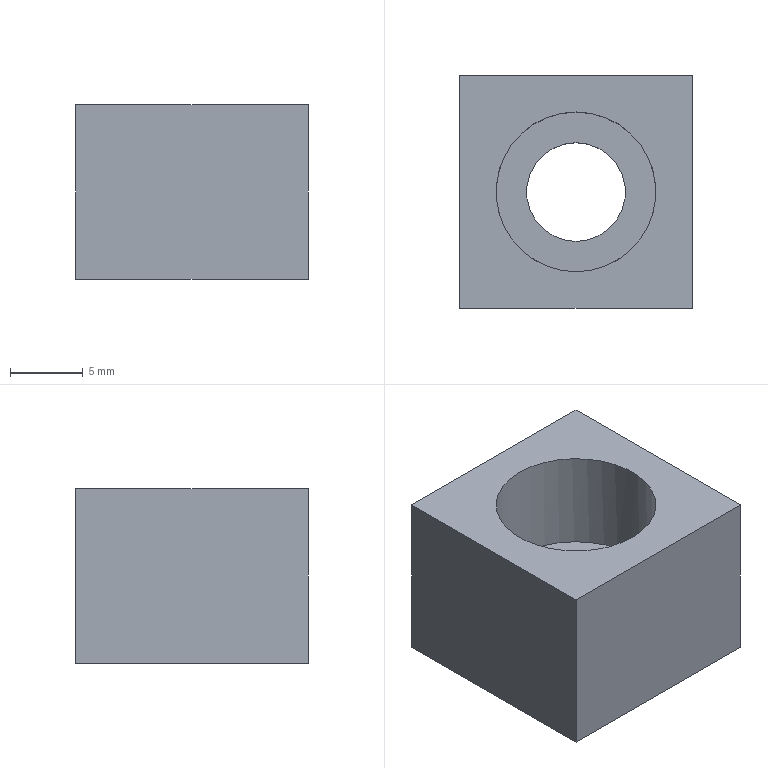Part | STEP file | lll_id62_x_t | 1 solid | 75 faces | box 16 x 16 x 12 mm | volume 2222 mm3 | plane 55 | other 18 | cylinder 2 | commonest cylinder face diameters 6.8 x1 11 x1